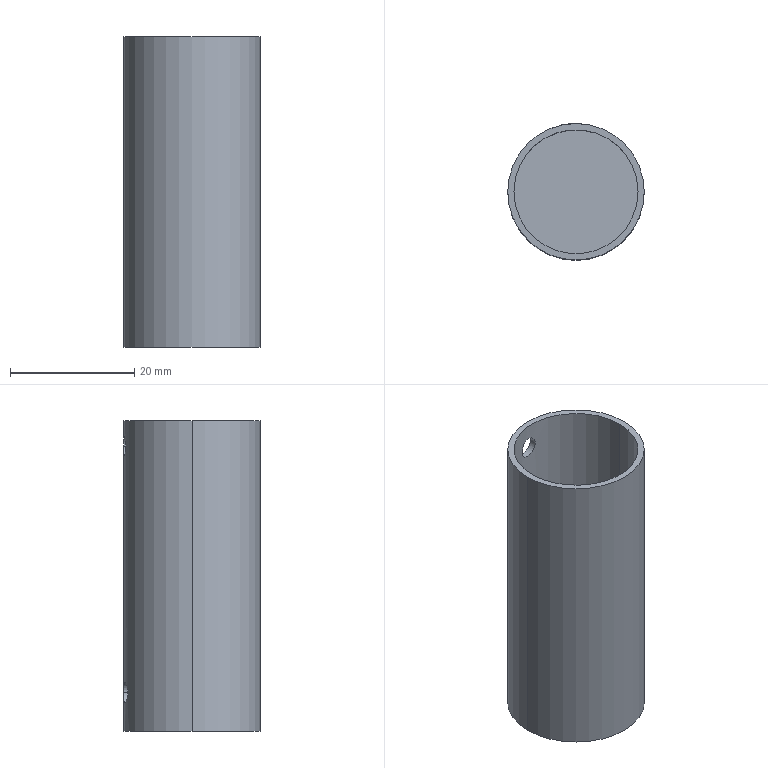Part | NX | 1 solid | 14 faces | box 22 x 22 x 50 mm | volume 4852 mm3 | cylinder 10 | plane 4 | commonest cylinder face diameters 3.3 x4 20 x4 22 x2
STEP:
#1=CARTESIAN_POINT('',(-0.2065,9.998,6.201));
#2=VERTEX_POINT('',#1);
#3=CARTESIAN_POINT('',(-3.449,9.386,6.201));
#4=VERTEX_POINT('',#3);
#5=CARTESIAN_POINT('',(-0.2065,9.998,6.201));
#6=CARTESIAN_POINT('',(-0.2065,9.998,6.018));
#7=CARTESIAN_POINT('',(-0.2384,9.997,5.832));
#8=CARTESIAN_POINT('',(-0.2992,9.996,5.659));
#9=CARTESIAN_POINT('',(-0.3601,9.994,5.486));
#10=CARTESIAN_POINT('',(-0.4514,9.99,5.322));
#11=CARTESIAN_POINT('',(-0.5654,9.984,5.178));
#12=CARTESIAN_POINT('',(-0.6803,9.977,5.034));
#13=CARTESIAN_POINT('',(-0.8214,9.967,4.907));
#14=CARTESIAN_POINT('',(-0.9768,9.952,4.808));
#15=CARTESIAN_POINT('',(-1.133,9.937,4.709));
#16=CARTESIAN_POINT('',(-1.308,9.916,4.635));
#17=CARTESIAN_POINT('',(-1.487,9.889,4.593));
#18=CARTESIAN_POINT('',(-1.665,9.862,4.552));
#19=CARTESIAN_POINT('',(-1.851,9.829,4.541));
#20=CARTESIAN_POINT('',(-2.03,9.792,4.561));
#21=CARTESIAN_POINT('',(-2.208,9.755,4.581));
#22=CARTESIAN_POINT('',(-2.383,9.713,4.632));
#23=CARTESIAN_POINT('',(-2.543,9.671,4.71));
#24=CARTESIAN_POINT('',(-2.703,9.629,4.788));
#25=CARTESIAN_POINT('',(-2.851,9.586,4.895));
#26=CARTESIAN_POINT('',(-2.977,9.547,5.023));
#27=CARTESIAN_POINT('',(-3.103,9.507,5.153));
#28=CARTESIAN_POINT('',(-3.21,9.471,5.307));
#29=CARTESIAN_POINT('',(-3.288,9.444,5.473));
#30=CARTESIAN_POINT('',(-3.366,9.417,5.639));
#31=CARTESIAN_POINT('',(-3.417,9.398,5.822));
#32=CARTESIAN_POINT('',(-3.438,9.39,6.006));
#33=CARTESIAN_POINT('',(-3.446,9.388,6.071));
#34=CARTESIAN_POINT('',(-3.449,9.386,6.136));
#35=CARTESIAN_POINT('',(-3.449,9.386,6.201));
#36=B_SPLINE_CURVE_WITH_KNOTS('',3,(#5,#6,#7,#8,#9,#10,#11,#12,#13,#14,#15,#16,#17,#18,#19,#20,#21,#22,#23,#24,#25,#26,#27,#28,#29,#30,#31,#32,#33,#34,#35),.UNSPECIFIED.,.F.,.F.,(4,3,3,3,3,3,3,3,3,3,4),(0.,0.1064,0.2128,0.3201,0.428,0.535,0.6409,0.7472,0.8549,0.9627,1.),.UNSPECIFIED.);
#37=EDGE_CURVE('',#2,#4,#36,.T.);
#38=ORIENTED_EDGE('',*,*,#37,.F.);
#39=CARTESIAN_POINT('',(-0.3942,10.993,6.201));
#40=VERTEX_POINT('',#39);
#41=CARTESIAN_POINT('',(-0.4173,11.115,6.201));
#42=DIRECTION('',(0.1853,-0.9827,0.));
#43=VECTOR('',#42,1.);
#44=LINE('',#41,#43);
#45=EDGE_CURVE('',#40,#2,#44,.T.);
#46=ORIENTED_EDGE('',*,*,#45,.F.);
#47=CARTESIAN_POINT('',(-3.637,10.381,6.201));
#48=VERTEX_POINT('',#47);
#49=CARTESIAN_POINT('',(-3.637,10.381,6.201));
#50=CARTESIAN_POINT('',(-3.637,10.381,6.017));
#51=CARTESIAN_POINT('',(-3.607,10.392,5.831));
#52=CARTESIAN_POINT('',(-3.549,10.412,5.658));
#53=CARTESIAN_POINT('',(-3.492,10.431,5.485));
#54=CARTESIAN_POINT('',(-3.405,10.46,5.32));
#55=CARTESIAN_POINT('',(-3.296,10.495,5.177));
#56=CARTESIAN_POINT('',(-3.186,10.529,5.032));
#57=CARTESIAN_POINT('',(-3.05,10.57,4.906));
#58=CARTESIAN_POINT('',(-2.9,10.611,4.807));
#59=CARTESIAN_POINT('',(-2.748,10.652,4.708));
#60=CARTESIAN_POINT('',(-2.577,10.695,4.634));
#61=CARTESIAN_POINT('',(-2.401,10.735,4.593));
#62=CARTESIAN_POINT('',(-2.226,10.774,4.552));
#63=CARTESIAN_POINT('',(-2.04,10.811,4.541));
#64=CARTESIAN_POINT('',(-1.859,10.842,4.561));
#65=CARTESIAN_POINT('',(-1.68,10.872,4.581));
#66=CARTESIAN_POINT('',(-1.501,10.898,4.633));
#67=CARTESIAN_POINT('',(-1.338,10.918,4.711));
#68=CARTESIAN_POINT('',(-1.173,10.939,4.79));
#69=CARTESIAN_POINT('',(-1.019,10.953,4.898));
#70=CARTESIAN_POINT('',(-0.8887,10.964,5.026));
#71=CARTESIAN_POINT('',(-0.7569,10.975,5.156));
#72=CARTESIAN_POINT('',(-0.6452,10.981,5.31));
#73=CARTESIAN_POINT('',(-0.5634,10.986,5.476));
#74=CARTESIAN_POINT('',(-0.4815,10.99,5.643));
#75=CARTESIAN_POINT('',(-0.4272,10.992,5.826));
#76=CARTESIAN_POINT('',(-0.4055,10.993,6.01));
#77=CARTESIAN_POINT('',(-0.398,10.993,6.073));
#78=CARTESIAN_POINT('',(-0.3942,10.993,6.137));
#79=CARTESIAN_POINT('',(-0.3942,10.993,6.201));
#80=B_SPLINE_CURVE_WITH_KNOTS('',3,(#49,#50,#51,#52,#53,#54,#55,#56,#57,#58,#59,#60,#61,#62,#63,#64,#65,#66,#67,#68,#69,#70,#71,#72,#73,#74,#75,#76,#77,#78,#79),.UNSPECIFIED.,.F.,.F.,(4,3,3,3,3,3,3,3,3,3,4),(0.,0.1066,0.2131,0.3205,0.4283,0.5353,0.6415,0.748,0.8557,0.9634,1.),.UNSPECIFIED.);
#81=EDGE_CURVE('',#48,#40,#80,.T.);
#82=ORIENTED_EDGE('',*,*,#81,.F.);
#83=CARTESIAN_POINT('',(-3.66,10.504,6.201));
#84=DIRECTION('',(0.1853,-0.9827,0.));
#85=VECTOR('',#84,1.);
#86=LINE('',#83,#85);
#87=EDGE_CURVE('',#48,#4,#86,.T.);
#88=ORIENTED_EDGE('',*,*,#87,.T.);
#89=EDGE_LOOP('',(#38,#46,#82,#88));
#90=FACE_OUTER_BOUND('',#89,.T.);
#91=CARTESIAN_POINT('',(-2.039,10.809,6.201));
#92=DIRECTION('',(-0.1853,0.9827,0.));
#93=DIRECTION('',(-0.9827,-0.1853,0.));
#94=AXIS2_PLACEMENT_3D('',#91,#92,#93);
#95=CYLINDRICAL_SURFACE('',#94,1.65);
#96=ADVANCED_FACE('',(#90),#95,.F.);
#97=CARTESIAN_POINT('',(0.6601,9.978,45.914));
#98=VERTEX_POINT('',#97);
#99=CARTESIAN_POINT('',(-2.624,9.65,45.914));
#100=VERTEX_POINT('',#99);
#101=CARTESIAN_POINT('',(0.6601,9.978,45.914));
#102=CARTESIAN_POINT('',(0.6601,9.978,45.731));
#103=CARTESIAN_POINT('',(0.6283,9.98,45.545));
#104=CARTESIAN_POINT('',(0.5675,9.984,45.372));
#105=CARTESIAN_POINT('',(0.5068,9.987,45.199));
#106=CARTESIAN_POINT('',(0.4155,9.992,45.034));
#107=CARTESIAN_POINT('',(0.3014,9.995,44.891));
#108=CARTESIAN_POINT('',(0.1863,9.999,44.747));
#109=CARTESIAN_POINT('',(0.0449,10.001,44.62));
#110=CARTESIAN_POINT('',(-0.1113,9.999,44.521));
#111=CARTESIAN_POINT('',(-0.2683,9.998,44.422));
#112=CARTESIAN_POINT('',(-0.4446,9.992,44.348));
#113=CARTESIAN_POINT('',(-0.6254,9.98,44.306));
#114=CARTESIAN_POINT('',(-0.8044,9.969,44.265));
#115=CARTESIAN_POINT('',(-0.9928,9.952,44.254));
#116=CARTESIAN_POINT('',(-1.175,9.931,44.274));
#117=CARTESIAN_POINT('',(-1.355,9.909,44.294));
#118=CARTESIAN_POINT('',(-1.533,9.883,44.345));
#119=CARTESIAN_POINT('',(-1.696,9.855,44.423));
#120=CARTESIAN_POINT('',(-1.859,9.827,44.501));
#121=CARTESIAN_POINT('',(-2.011,9.797,44.608));
#122=CARTESIAN_POINT('',(-2.139,9.769,44.736));
#123=CARTESIAN_POINT('',(-2.268,9.74,44.866));
#124=CARTESIAN_POINT('',(-2.378,9.714,45.02));
#125=CARTESIAN_POINT('',(-2.458,9.693,45.186));
#126=CARTESIAN_POINT('',(-2.538,9.673,45.352));
#127=CARTESIAN_POINT('',(-2.591,9.659,45.535));
#128=CARTESIAN_POINT('',(-2.612,9.653,45.719));
#129=CARTESIAN_POINT('',(-2.62,9.651,45.784));
#130=CARTESIAN_POINT('',(-2.624,9.65,45.849));
#131=CARTESIAN_POINT('',(-2.624,9.65,45.914));
#132=B_SPLINE_CURVE_WITH_KNOTS('',3,(#101,#102,#103,#104,#105,#106,#107,#108,#109,#110,#111,#112,#113,#114,#115,#116,#117,#118,#119,#120,#121,#122,#123,#124,#125,#126,#127,#128,#129,#130,#131),.UNSPECIFIED.,.F.,.F.,(4,3,3,3,3,3,3,3,3,3,4),(0.,0.1064,0.2128,0.3201,0.428,0.535,0.6409,0.7472,0.8549,0.9627,1.),.UNSPECIFIED.);
#133=EDGE_CURVE('',#98,#100,#132,.T.);
#134=ORIENTED_EDGE('',*,*,#133,.F.);
#135=CARTESIAN_POINT('',(0.5593,10.986,45.914));
#136=VERTEX_POINT('',#135);
#137=CARTESIAN_POINT('',(0.5469,11.11,45.914));
#138=DIRECTION('',(0.09954,-0.995,0.));
#139=VECTOR('',#138,1.);
#140=LINE('',#137,#139);
#141=EDGE_CURVE('',#136,#98,#140,.T.);
#142=ORIENTED_EDGE('',*,*,#141,.F.);
#143=CARTESIAN_POINT('',(-2.724,10.657,45.914));
#144=VERTEX_POINT('',#143);
#145=CARTESIAN_POINT('',(-2.724,10.657,45.914));
#146=CARTESIAN_POINT('',(-2.724,10.657,45.73));
#147=CARTESIAN_POINT('',(-2.693,10.665,45.544));
#148=CARTESIAN_POINT('',(-2.634,10.68,45.371));
#149=CARTESIAN_POINT('',(-2.575,10.694,45.198));
#150=CARTESIAN_POINT('',(-2.486,10.716,45.033));
#151=CARTESIAN_POINT('',(-2.375,10.741,44.89));
#152=CARTESIAN_POINT('',(-2.262,10.766,44.745));
#153=CARTESIAN_POINT('',(-2.124,10.794,44.619));
#154=CARTESIAN_POINT('',(-1.97,10.822,44.52));
#155=CARTESIAN_POINT('',(-1.815,10.85,44.421));
#156=CARTESIAN_POINT('',(-1.641,10.878,44.347));
#157=CARTESIAN_POINT('',(-1.462,10.902,44.306));
#158=CARTESIAN_POINT('',(-1.284,10.926,44.265));
#159=CARTESIAN_POINT('',(-1.096,10.947,44.254));
#160=CARTESIAN_POINT('',(-0.9135,10.962,44.274));
#161=CARTESIAN_POINT('',(-0.7325,10.977,44.294));
#162=CARTESIAN_POINT('',(-0.552,10.987,44.346));
#163=CARTESIAN_POINT('',(-0.387,10.993,44.424));
#164=CARTESIAN_POINT('',(-0.2214,10.999,44.503));
#165=CARTESIAN_POINT('',(-0.06681,11.001,44.611));
#166=CARTESIAN_POINT('',(0.06417,11.,44.739));
#167=CARTESIAN_POINT('',(0.1964,10.999,44.869));
#168=CARTESIAN_POINT('',(0.3082,10.996,45.023));
#169=CARTESIAN_POINT('',(0.3901,10.993,45.189));
#170=CARTESIAN_POINT('',(0.4721,10.99,45.356));
#171=CARTESIAN_POINT('',(0.5264,10.987,45.539));
#172=CARTESIAN_POINT('',(0.5481,10.986,45.723));
#173=CARTESIAN_POINT('',(0.5555,10.986,45.786));
#174=CARTESIAN_POINT('',(0.5593,10.986,45.85));
#175=CARTESIAN_POINT('',(0.5593,10.986,45.914));
#176=B_SPLINE_CURVE_WITH_KNOTS('',3,(#145,#146,#147,#148,#149,#150,#151,#152,#153,#154,#155,#156,#157,#158,#159,#160,#161,#162,#163,#164,#165,#166,#167,#168,#169,#170,#171,#172,#173,#174,#175),.UNSPECIFIED.,.F.,.F.,(4,3,3,3,3,3,3,3,3,3,4),(0.,0.1066,0.2131,0.3205,0.4283,0.5353,0.6415,0.748,0.8557,0.9634,1.),.UNSPECIFIED.);
#177=EDGE_CURVE('',#144,#136,#176,.T.);
#178=ORIENTED_EDGE('',*,*,#177,.F.);
#179=CARTESIAN_POINT('',(-2.737,10.781,45.914));
#180=DIRECTION('',(0.09954,-0.995,0.));
#181=VECTOR('',#180,1.);
#182=LINE('',#179,#181);
#183=EDGE_CURVE('',#144,#100,#182,.T.);
#184=ORIENTED_EDGE('',*,*,#183,.T.);
#185=EDGE_LOOP('',(#134,#142,#178,#184));
#186=FACE_OUTER_BOUND('',#185,.T.);
#187=CARTESIAN_POINT('',(-1.095,10.945,45.914));
#188=DIRECTION('',(-0.09954,0.995,0.));
#189=DIRECTION('',(-0.995,-0.09954,0.));
#190=AXIS2_PLACEMENT_3D('',#187,#188,#189);
#191=CYLINDRICAL_SURFACE('',#190,1.65);
#192=ADVANCED_FACE('',(#186),#191,.F.);
#193=CARTESIAN_POINT('',(10.,0.,25.));
#194=VERTEX_POINT('',#193);
#195=CARTESIAN_POINT('',(-10.,0.,25.));
#196=VERTEX_POINT('',#195);
#197=CARTESIAN_POINT('',(0.,0.,25.));
#198=DIRECTION('',(0.,0.,-1.));
#199=DIRECTION('',(-1.,0.,0.));
#200=AXIS2_PLACEMENT_3D('',#197,#198,#199);
#201=CIRCLE('',#200,10.);
#202=EDGE_CURVE('',#194,#196,#201,.T.);
#203=ORIENTED_EDGE('',*,*,#202,.F.);
#204=CARTESIAN_POINT('',(10.,0.,0.));
#205=VERTEX_POINT('',#204);
#206=CARTESIAN_POINT('',(10.,0.,25.));
#207=DIRECTION('',(0.,0.,1.));
#208=VECTOR('',#207,1.);
#209=LINE('',#206,#208);
#210=EDGE_CURVE('',#205,#194,#209,.T.);
#211=ORIENTED_EDGE('',*,*,#210,.F.);
#212=CARTESIAN_POINT('',(-10.,0.,0.));
#213=VERTEX_POINT('',#212);
#214=CARTESIAN_POINT('',(0.,0.,0.));
#215=DIRECTION('',(0.,0.,-1.));
#216=DIRECTION('',(-1.,0.,0.));
#217=AXIS2_PLACEMENT_3D('',#214,#215,#216);
#218=CIRCLE('',#217,10.);
#219=EDGE_CURVE('',#205,#213,#218,.T.);
#220=ORIENTED_EDGE('',*,*,#219,.T.);
#221=CARTESIAN_POINT('',(-10.,0.,25.));
#222=DIRECTION('',(0.,0.,1.));
#223=VECTOR('',#222,1.);
#224=LINE('',#221,#223);
#225=EDGE_CURVE('',#213,#196,#224,.T.);
#226=ORIENTED_EDGE('',*,*,#225,.T.);
#227=EDGE_LOOP('',(#203,#211,#220,#226));
#228=FACE_OUTER_BOUND('',#227,.T.);
#229=CARTESIAN_POINT('',(0.,0.,25.));
#230=DIRECTION('',(0.,0.,-1.));
#231=DIRECTION('',(-1.,0.,0.));
#232=AXIS2_PLACEMENT_3D('',#229,#230,#231);
#233=CYLINDRICAL_SURFACE('',#232,10.);
#234=ADVANCED_FACE('',(#228),#233,.F.);
#235=CARTESIAN_POINT('',(-10.,0.,30.));
#236=VERTEX_POINT('',#235);
#237=CARTESIAN_POINT('',(10.,0.,30.));
#238=VERTEX_POINT('',#237);
#239=CARTESIAN_POINT('',(0.,0.,30.));
#240=DIRECTION('',(0.,0.,1.));
#241=DIRECTION('',(1.,0.,0.));
#242=AXIS2_PLACEMENT_3D('',#239,#240,#241);
#243=CIRCLE('',#242,10.);
#244=EDGE_CURVE('',#236,#238,#243,.T.);
#245=ORIENTED_EDGE('',*,*,#244,.F.);
#246=CARTESIAN_POINT('',(-10.,0.,50.));
#247=VERTEX_POINT('',#246);
#248=CARTESIAN_POINT('',(-10.,0.,30.));
#249=DIRECTION('',(0.,0.,1.));
#250=VECTOR('',#249,1.);
#251=LINE('',#248,#250);
#252=EDGE_CURVE('',#236,#247,#251,.T.);
#253=ORIENTED_EDGE('',*,*,#252,.T.);
#254=CARTESIAN_POINT('',(10.,0.,50.));
#255=VERTEX_POINT('',#254);
#256=CARTESIAN_POINT('',(0.,0.,50.));
#257=DIRECTION('',(0.,0.,1.));
#258=DIRECTION('',(1.,0.,0.));
#259=AXIS2_PLACEMENT_3D('',#256,#257,#258);
#260=CIRCLE('',#259,10.);
#261=EDGE_CURVE('',#247,#255,#260,.T.);
#262=ORIENTED_EDGE('',*,*,#261,.T.);
#263=CARTESIAN_POINT('',(10.,0.,30.));
#264=DIRECTION('',(0.,0.,1.));
#265=VECTOR('',#264,1.);
#266=LINE('',#263,#265);
#267=EDGE_CURVE('',#238,#255,#266,.T.);
#268=ORIENTED_EDGE('',*,*,#267,.F.);
#269=EDGE_LOOP('',(#245,#253,#262,#268));
#270=FACE_OUTER_BOUND('',#269,.T.);
#271=CARTESIAN_POINT('',(0.,0.,30.));
#272=DIRECTION('',(0.,0.,1.));
#273=DIRECTION('',(1.,0.,0.));
#274=AXIS2_PLACEMENT_3D('',#271,#272,#273);
#275=CYLINDRICAL_SURFACE('',#274,10.);
#276=ADVANCED_FACE('',(#270),#275,.F.);
#277=ORIENTED_EDGE('',*,*,#81,.T.);
#278=CARTESIAN_POINT('',(-0.3942,10.993,6.201));
#279=CARTESIAN_POINT('',(-0.3942,10.993,6.385));
#280=CARTESIAN_POINT('',(-0.4261,10.992,6.571));
#281=CARTESIAN_POINT('',(-0.4869,10.989,6.744));
#282=CARTESIAN_POINT('',(-0.5477,10.987,6.917));
#283=CARTESIAN_POINT('',(-0.6391,10.982,7.082));
#284=CARTESIAN_POINT('',(-0.7532,10.974,7.225));
#285=CARTESIAN_POINT('',(-0.8681,10.966,7.37));
#286=CARTESIAN_POINT('',(-1.009,10.955,7.496));
#287=CARTESIAN_POINT('',(-1.165,10.938,7.595));
#288=CARTESIAN_POINT('',(-1.321,10.922,7.694));
#289=CARTESIAN_POINT('',(-1.496,10.899,7.768));
#290=CARTESIAN_POINT('',(-1.674,10.872,7.809));
#291=CARTESIAN_POINT('',(-1.852,10.844,7.85));
#292=CARTESIAN_POINT('',(-2.038,10.811,7.861));
#293=CARTESIAN_POINT('',(-2.217,10.774,7.841));
#294=CARTESIAN_POINT('',(-2.395,10.738,7.821));
#295=CARTESIAN_POINT('',(-2.571,10.697,7.769));
#296=CARTESIAN_POINT('',(-2.731,10.656,7.691));
#297=CARTESIAN_POINT('',(-2.892,10.614,7.612));
#298=CARTESIAN_POINT('',(-3.041,10.572,7.504));
#299=CARTESIAN_POINT('',(-3.166,10.535,7.376));
#300=CARTESIAN_POINT('',(-3.293,10.496,7.246));
#301=CARTESIAN_POINT('',(-3.399,10.462,7.092));
#302=CARTESIAN_POINT('',(-3.477,10.436,6.926));
#303=CARTESIAN_POINT('',(-3.555,10.41,6.759));
#304=CARTESIAN_POINT('',(-3.606,10.392,6.576));
#305=CARTESIAN_POINT('',(-3.626,10.385,6.392));
#306=CARTESIAN_POINT('',(-3.633,10.383,6.329));
#307=CARTESIAN_POINT('',(-3.637,10.381,6.265));
#308=CARTESIAN_POINT('',(-3.637,10.381,6.201));
#309=B_SPLINE_CURVE_WITH_KNOTS('',3,(#278,#279,#280,#281,#282,#283,#284,#285,#286,#287,#288,#289,#290,#291,#292,#293,#294,#295,#296,#297,#298,#299,#300,#301,#302,#303,#304,#305,#306,#307,#308),.UNSPECIFIED.,.F.,.F.,(4,3,3,3,3,3,3,3,3,3,4),(0.,0.1066,0.2131,0.3205,0.4283,0.5353,0.6415,0.748,0.8557,0.9634,1.),.UNSPECIFIED.);
#310=EDGE_CURVE('',#40,#48,#309,.T.);
#311=ORIENTED_EDGE('',*,*,#310,.T.);
#312=EDGE_LOOP('',(#277,#311));
#313=FACE_BOUND('',#312,.T.);
#314=ORIENTED_EDGE('',*,*,#177,.T.);
#315=CARTESIAN_POINT('',(0.5593,10.986,45.914));
#316=CARTESIAN_POINT('',(0.5593,10.986,46.097));
#317=CARTESIAN_POINT('',(0.5275,10.988,46.283));
#318=CARTESIAN_POINT('',(0.4666,10.99,46.457));
#319=CARTESIAN_POINT('',(0.4058,10.993,46.63));
#320=CARTESIAN_POINT('',(0.3143,10.996,46.795));
#321=CARTESIAN_POINT('',(0.2,10.998,46.938));
#322=CARTESIAN_POINT('',(0.08485,11.,47.082));
#323=CARTESIAN_POINT('',(-0.05668,11.001,47.209));
#324=CARTESIAN_POINT('',(-0.2129,10.998,47.308));
#325=CARTESIAN_POINT('',(-0.3698,10.995,47.407));
#326=CARTESIAN_POINT('',(-0.546,10.988,47.48));
#327=CARTESIAN_POINT('',(-0.7265,10.976,47.522));
#328=CARTESIAN_POINT('',(-0.9057,10.964,47.563));
#329=CARTESIAN_POINT('',(-1.094,10.947,47.574));
#330=CARTESIAN_POINT('',(-1.276,10.926,47.554));
#331=CARTESIAN_POINT('',(-1.456,10.905,47.534));
#332=CARTESIAN_POINT('',(-1.635,10.879,47.482));
#333=CARTESIAN_POINT('',(-1.798,10.852,47.404));
#334=CARTESIAN_POINT('',(-1.962,10.825,47.325));
#335=CARTESIAN_POINT('',(-2.114,10.796,47.217));
#336=CARTESIAN_POINT('',(-2.242,10.769,47.089));
#337=CARTESIAN_POINT('',(-2.371,10.742,46.959));
#338=CARTESIAN_POINT('',(-2.48,10.717,46.805));
#339=CARTESIAN_POINT('',(-2.56,10.698,46.638));
#340=CARTESIAN_POINT('',(-2.64,10.679,46.472));
#341=CARTESIAN_POINT('',(-2.692,10.665,46.289));
#342=CARTESIAN_POINT('',(-2.713,10.66,46.105));
#343=CARTESIAN_POINT('',(-2.721,10.658,46.042));
#344=CARTESIAN_POINT('',(-2.724,10.657,45.978));
#345=CARTESIAN_POINT('',(-2.724,10.657,45.914));
#346=B_SPLINE_CURVE_WITH_KNOTS('',3,(#315,#316,#317,#318,#319,#320,#321,#322,#323,#324,#325,#326,#327,#328,#329,#330,#331,#332,#333,#334,#335,#336,#337,#338,#339,#340,#341,#342,#343,#344,#345),.UNSPECIFIED.,.F.,.F.,(4,3,3,3,3,3,3,3,3,3,4),(0.,0.1066,0.2131,0.3205,0.4283,0.5353,0.6415,0.748,0.8557,0.9634,1.),.UNSPECIFIED.);
#347=EDGE_CURVE('',#136,#144,#346,.T.);
#348=ORIENTED_EDGE('',*,*,#347,.T.);
#349=EDGE_LOOP('',(#314,#348));
#350=FACE_BOUND('',#349,.T.);
#351=CARTESIAN_POINT('',(11.,0.,50.));
#352=VERTEX_POINT('',#351);
#353=CARTESIAN_POINT('',(-11.,0.,50.));
#354=VERTEX_POINT('',#353);
#355=CARTESIAN_POINT('',(0.,0.,50.));
#356=DIRECTION('',(0.,0.,1.));
#357=DIRECTION('',(1.,0.,0.));
#358=AXIS2_PLACEMENT_3D('',#355,#356,#357);
#359=CIRCLE('',#358,11.);
#360=EDGE_CURVE('',#352,#354,#359,.T.);
#361=ORIENTED_EDGE('',*,*,#360,.F.);
#362=CARTESIAN_POINT('',(11.,0.,0.));
#363=VERTEX_POINT('',#362);
#364=CARTESIAN_POINT('',(11.,0.,50.));
#365=DIRECTION('',(0.,0.,1.));
#366=VECTOR('',#365,1.);
#367=LINE('',#364,#366);
#368=EDGE_CURVE('',#363,#352,#367,.T.);
#369=ORIENTED_EDGE('',*,*,#368,.F.);
#370=CARTESIAN_POINT('',(-11.,0.,0.));
#371=VERTEX_POINT('',#370);
#372=CARTESIAN_POINT('',(0.,0.,0.));
#373=DIRECTION('',(0.,0.,1.));
#374=DIRECTION('',(1.,0.,0.));
#375=AXIS2_PLACEMENT_3D('',#372,#373,#374);
#376=CIRCLE('',#375,11.);
#377=EDGE_CURVE('',#363,#371,#376,.T.);
#378=ORIENTED_EDGE('',*,*,#377,.T.);
#379=CARTESIAN_POINT('',(-11.,0.,50.));
#380=DIRECTION('',(0.,0.,1.));
#381=VECTOR('',#380,1.);
#382=LINE('',#379,#381);
#383=EDGE_CURVE('',#371,#354,#382,.T.);
#384=ORIENTED_EDGE('',*,*,#383,.T.);
#385=EDGE_LOOP('',(#361,#369,#378,#384));
#386=FACE_BOUND('',#385,.T.);
#387=CARTESIAN_POINT('',(0.,0.,50.));
#388=DIRECTION('',(0.,0.,-1.));
#389=DIRECTION('',(-1.,0.,0.));
#390=AXIS2_PLACEMENT_3D('',#387,#388,#389);
#391=CYLINDRICAL_SURFACE('',#390,11.);
#392=ADVANCED_FACE('',(#313,#350,#386),#391,.T.);
#393=ORIENTED_EDGE('',*,*,#368,.T.);
#394=CARTESIAN_POINT('',(0.,0.,50.));
#395=DIRECTION('',(0.,0.,1.));
#396=DIRECTION('',(1.,0.,0.));
#397=AXIS2_PLACEMENT_3D('',#394,#395,#396);
#398=CIRCLE('',#397,11.);
#399=EDGE_CURVE('',#354,#352,#398,.T.);
#400=ORIENTED_EDGE('',*,*,#399,.F.);
#401=ORIENTED_EDGE('',*,*,#383,.F.);
#402=CARTESIAN_POINT('',(0.,0.,0.));
#403=DIRECTION('',(0.,0.,1.));
#404=DIRECTION('',(1.,0.,0.));
#405=AXIS2_PLACEMENT_3D('',#402,#403,#404);
#406=CIRCLE('',#405,11.);
#407=EDGE_CURVE('',#371,#363,#406,.T.);
#408=ORIENTED_EDGE('',*,*,#407,.T.);
#409=EDGE_LOOP('',(#393,#400,#401,#408));
#410=FACE_OUTER_BOUND('',#409,.T.);
#411=CARTESIAN_POINT('',(0.,0.,50.));
#412=DIRECTION('',(0.,0.,-1.));
#413=DIRECTION('',(-1.,0.,0.));
#414=AXIS2_PLACEMENT_3D('',#411,#412,#413);
#415=CYLINDRICAL_SURFACE('',#414,11.);
#416=ADVANCED_FACE('',(#410),#415,.T.);
#417=CARTESIAN_POINT('',(0.,0.,50.));
#418=DIRECTION('',(0.,0.,1.));
#419=DIRECTION('',(1.,0.,0.));
#420=AXIS2_PLACEMENT_3D('',#417,#418,#419);
#421=CIRCLE('',#420,10.);
#422=EDGE_CURVE('',#255,#247,#421,.T.);
#423=ORIENTED_EDGE('',*,*,#422,.F.);
#424=ORIENTED_EDGE('',*,*,#261,.F.);
#425=EDGE_LOOP('',(#423,#424));
#426=FACE_BOUND('',#425,.T.);
#427=ORIENTED_EDGE('',*,*,#399,.T.);
#428=ORIENTED_EDGE('',*,*,#360,.T.);
#429=EDGE_LOOP('',(#427,#428));
#430=FACE_BOUND('',#429,.T.);
#431=CARTESIAN_POINT('',(0.,0.,50.));
#432=DIRECTION('',(0.,0.,1.));
#433=DIRECTION('',(1.,0.,0.));
#434=AXIS2_PLACEMENT_3D('',#431,#432,#433);
#435=PLANE('',#434);
#436=ADVANCED_FACE('',(#426,#430),#435,.T.);
#437=CARTESIAN_POINT('',(0.,0.,0.));
#438=DIRECTION('',(0.,0.,-1.));
#439=DIRECTION('',(-1.,0.,0.));
#440=AXIS2_PLACEMENT_3D('',#437,#438,#439);
#441=CIRCLE('',#440,10.);
#442=EDGE_CURVE('',#213,#205,#441,.T.);
#443=ORIENTED_EDGE('',*,*,#442,.F.);
#444=ORIENTED_EDGE('',*,*,#219,.F.);
#445=EDGE_LOOP('',(#443,#444));
#446=FACE_BOUND('',#445,.T.);
#447=ORIENTED_EDGE('',*,*,#407,.F.);
#448=ORIENTED_EDGE('',*,*,#377,.F.);
#449=EDGE_LOOP('',(#447,#448));
#450=FACE_BOUND('',#449,.T.);
#451=CARTESIAN_POINT('',(0.,0.,0.));
#452=DIRECTION('',(0.,0.,1.));
#453=DIRECTION('',(1.,0.,0.));
#454=AXIS2_PLACEMENT_3D('',#451,#452,#453);
#455=PLANE('',#454);
#456=ADVANCED_FACE('',(#446,#450),#455,.F.);
#457=ORIENTED_EDGE('',*,*,#252,.F.);
#458=CARTESIAN_POINT('',(0.,0.,30.));
#459=DIRECTION('',(0.,0.,1.));
#460=DIRECTION('',(1.,0.,0.));
#461=AXIS2_PLACEMENT_3D('',#458,#459,#460);
#462=CIRCLE('',#461,10.);
#463=EDGE_CURVE('',#238,#236,#462,.T.);
#464=ORIENTED_EDGE('',*,*,#463,.F.);
#465=ORIENTED_EDGE('',*,*,#267,.T.);
#466=ORIENTED_EDGE('',*,*,#422,.T.);
#467=EDGE_LOOP('',(#457,#464,#465,#466));
#468=FACE_BOUND('',#467,.T.);
#469=CARTESIAN_POINT('',(-2.624,9.65,45.914));
#470=CARTESIAN_POINT('',(-2.624,9.65,46.097));
#471=CARTESIAN_POINT('',(-2.593,9.658,46.283));
#472=CARTESIAN_POINT('',(-2.534,9.674,46.456));
#473=CARTESIAN_POINT('',(-2.475,9.689,46.629));
#474=CARTESIAN_POINT('',(-2.387,9.712,46.793));
#475=CARTESIAN_POINT('',(-2.275,9.738,46.937));
#476=CARTESIAN_POINT('',(-2.163,9.764,47.081));
#477=CARTESIAN_POINT('',(-2.025,9.794,47.208));
#478=CARTESIAN_POINT('',(-1.872,9.823,47.307));
#479=CARTESIAN_POINT('',(-1.717,9.853,47.406));
#480=CARTESIAN_POINT('',(-1.543,9.882,47.48));
#481=CARTESIAN_POINT('',(-1.364,9.907,47.522));
#482=CARTESIAN_POINT('',(-1.186,9.931,47.563));
#483=CARTESIAN_POINT('',(-0.9982,9.952,47.574));
#484=CARTESIAN_POINT('',(-0.8158,9.967,47.554));
#485=CARTESIAN_POINT('',(-0.6351,9.981,47.534));
#486=CARTESIAN_POINT('',(-0.4549,9.991,47.483));
#487=CARTESIAN_POINT('',(-0.2901,9.996,47.405));
#488=CARTESIAN_POINT('',(-0.1245,10.001,47.327));
#489=CARTESIAN_POINT('',(0.03012,10.001,47.219));
#490=CARTESIAN_POINT('',(0.1613,9.999,47.092));
#491=CARTESIAN_POINT('',(0.294,9.997,46.962));
#492=CARTESIAN_POINT('',(0.4064,9.992,46.808));
#493=CARTESIAN_POINT('',(0.4888,9.988,46.642));
#494=CARTESIAN_POINT('',(0.5714,9.984,46.476));
#495=CARTESIAN_POINT('',(0.6262,9.98,46.293));
#496=CARTESIAN_POINT('',(0.6484,9.979,46.109));
#497=CARTESIAN_POINT('',(0.6562,9.978,46.044));
#498=CARTESIAN_POINT('',(0.6601,9.978,45.979));
#499=CARTESIAN_POINT('',(0.6601,9.978,45.914));
#500=B_SPLINE_CURVE_WITH_KNOTS('',3,(#469,#470,#471,#472,#473,#474,#475,#476,#477,#478,#479,#480,#481,#482,#483,#484,#485,#486,#487,#488,#489,#490,#491,#492,#493,#494,#495,#496,#497,#498,#499),.UNSPECIFIED.,.F.,.F.,(4,3,3,3,3,3,3,3,3,3,4),(0.,0.1064,0.2128,0.3201,0.428,0.535,0.6409,0.7472,0.8549,0.9627,1.),.UNSPECIFIED.);
#501=EDGE_CURVE('',#100,#98,#500,.T.);
#502=ORIENTED_EDGE('',*,*,#501,.T.);
#503=ORIENTED_EDGE('',*,*,#133,.T.);
#504=EDGE_LOOP('',(#502,#503));
#505=FACE_BOUND('',#504,.T.);
#506=CARTESIAN_POINT('',(0.,0.,30.));
#507=DIRECTION('',(0.,0.,1.));
#508=DIRECTION('',(1.,0.,0.));
#509=AXIS2_PLACEMENT_3D('',#506,#507,#508);
#510=CYLINDRICAL_SURFACE('',#509,10.);
#511=ADVANCED_FACE('',(#468,#505),#510,.F.);
#512=ORIENTED_EDGE('',*,*,#463,.T.);
#513=ORIENTED_EDGE('',*,*,#244,.T.);
#514=EDGE_LOOP('',(#512,#513));
#515=FACE_OUTER_BOUND('',#514,.T.);
#516=CARTESIAN_POINT('',(0.,0.,30.));
#517=DIRECTION('',(0.,0.,1.));
#518=DIRECTION('',(1.,0.,0.));
#519=AXIS2_PLACEMENT_3D('',#516,#517,#518);
#520=PLANE('',#519);
#521=ADVANCED_FACE('',(#515),#520,.T.);
#522=ORIENTED_EDGE('',*,*,#210,.T.);
#523=CARTESIAN_POINT('',(0.,0.,25.));
#524=DIRECTION('',(0.,0.,-1.));
#525=DIRECTION('',(-1.,0.,0.));
#526=AXIS2_PLACEMENT_3D('',#523,#524,#525);
#527=CIRCLE('',#526,10.);
#528=EDGE_CURVE('',#196,#194,#527,.T.);
#529=ORIENTED_EDGE('',*,*,#528,.F.);
#530=ORIENTED_EDGE('',*,*,#225,.F.);
#531=ORIENTED_EDGE('',*,*,#442,.T.);
#532=EDGE_LOOP('',(#522,#529,#530,#531));
#533=FACE_BOUND('',#532,.T.);
#534=CARTESIAN_POINT('',(-3.449,9.386,6.201));
#535=CARTESIAN_POINT('',(-3.449,9.386,6.384));
#536=CARTESIAN_POINT('',(-3.419,9.397,6.57));
#537=CARTESIAN_POINT('',(-3.362,9.418,6.743));
#538=CARTESIAN_POINT('',(-3.305,9.438,6.916));
#539=CARTESIAN_POINT('',(-3.219,9.469,7.08));
#540=CARTESIAN_POINT('',(-3.11,9.504,7.224));
#541=CARTESIAN_POINT('',(-3.001,9.54,7.368));
#542=CARTESIAN_POINT('',(-2.866,9.582,7.495));
#543=CARTESIAN_POINT('',(-2.715,9.624,7.594));
#544=CARTESIAN_POINT('',(-2.564,9.667,7.693));
#545=CARTESIAN_POINT('',(-2.393,9.711,7.767));
#546=CARTESIAN_POINT('',(-2.217,9.751,7.809));
#547=CARTESIAN_POINT('',(-2.042,9.791,7.85));
#548=CARTESIAN_POINT('',(-1.856,9.828,7.861));
#549=CARTESIAN_POINT('',(-1.676,9.859,7.841));
#550=CARTESIAN_POINT('',(-1.497,9.889,7.821));
#551=CARTESIAN_POINT('',(-1.318,9.914,7.77));
#552=CARTESIAN_POINT('',(-1.155,9.933,7.692));
#553=CARTESIAN_POINT('',(-0.9901,9.952,7.614));
#554=CARTESIAN_POINT('',(-0.8361,9.966,7.507));
#555=CARTESIAN_POINT('',(-0.7052,9.975,7.379));
#556=CARTESIAN_POINT('',(-0.5728,9.984,7.249));
#557=CARTESIAN_POINT('',(-0.4605,9.99,7.095));
#558=CARTESIAN_POINT('',(-0.378,9.993,6.929));
#559=CARTESIAN_POINT('',(-0.2954,9.996,6.763));
#560=CARTESIAN_POINT('',(-0.2405,9.997,6.58));
#561=CARTESIAN_POINT('',(-0.2183,9.998,6.396));
#562=CARTESIAN_POINT('',(-0.2105,9.998,6.331));
#563=CARTESIAN_POINT('',(-0.2065,9.998,6.266));
#564=CARTESIAN_POINT('',(-0.2065,9.998,6.201));
#565=B_SPLINE_CURVE_WITH_KNOTS('',3,(#534,#535,#536,#537,#538,#539,#540,#541,#542,#543,#544,#545,#546,#547,#548,#549,#550,#551,#552,#553,#554,#555,#556,#557,#558,#559,#560,#561,#562,#563,#564),.UNSPECIFIED.,.F.,.F.,(4,3,3,3,3,3,3,3,3,3,4),(0.,0.1064,0.2128,0.3201,0.428,0.535,0.6409,0.7472,0.8549,0.9627,1.),.UNSPECIFIED.);
#566=EDGE_CURVE('',#4,#2,#565,.T.);
#567=ORIENTED_EDGE('',*,*,#566,.T.);
#568=ORIENTED_EDGE('',*,*,#37,.T.);
#569=EDGE_LOOP('',(#567,#568));
#570=FACE_BOUND('',#569,.T.);
#571=CARTESIAN_POINT('',(0.,0.,25.));
#572=DIRECTION('',(0.,0.,-1.));
#573=DIRECTION('',(-1.,0.,0.));
#574=AXIS2_PLACEMENT_3D('',#571,#572,#573);
#575=CYLINDRICAL_SURFACE('',#574,10.);
#576=ADVANCED_FACE('',(#533,#570),#575,.F.);
#577=ORIENTED_EDGE('',*,*,#528,.T.);
#578=ORIENTED_EDGE('',*,*,#202,.T.);
#579=EDGE_LOOP('',(#577,#578));
#580=FACE_OUTER_BOUND('',#579,.T.);
#581=CARTESIAN_POINT('',(0.,0.,25.));
#582=DIRECTION('',(0.,0.,-1.));
#583=DIRECTION('',(-1.,0.,0.));
#584=AXIS2_PLACEMENT_3D('',#581,#582,#583);
#585=PLANE('',#584);
#586=ADVANCED_FACE('',(#580),#585,.T.);
#587=ORIENTED_EDGE('',*,*,#141,.T.);
#588=ORIENTED_EDGE('',*,*,#501,.F.);
#589=ORIENTED_EDGE('',*,*,#183,.F.);
#590=ORIENTED_EDGE('',*,*,#347,.F.);
#591=EDGE_LOOP('',(#587,#588,#589,#590));
#592=FACE_OUTER_BOUND('',#591,.T.);
#593=CARTESIAN_POINT('',(-1.095,10.945,45.914));
#594=DIRECTION('',(-0.09954,0.995,0.));
#595=DIRECTION('',(-0.995,-0.09954,0.));
#596=AXIS2_PLACEMENT_3D('',#593,#594,#595);
#597=CYLINDRICAL_SURFACE('',#596,1.65);
#598=ADVANCED_FACE('',(#592),#597,.F.);
#599=ORIENTED_EDGE('',*,*,#45,.T.);
#600=ORIENTED_EDGE('',*,*,#566,.F.);
#601=ORIENTED_EDGE('',*,*,#87,.F.);
#602=ORIENTED_EDGE('',*,*,#310,.F.);
#603=EDGE_LOOP('',(#599,#600,#601,#602));
#604=FACE_OUTER_BOUND('',#603,.T.);
#605=CARTESIAN_POINT('',(-2.039,10.809,6.201));
#606=DIRECTION('',(-0.1853,0.9827,0.));
#607=DIRECTION('',(-0.9827,-0.1853,0.));
#608=AXIS2_PLACEMENT_3D('',#605,#606,#607);
#609=CYLINDRICAL_SURFACE('',#608,1.65);
#610=ADVANCED_FACE('',(#604),#609,.F.);
#611=CLOSED_SHELL('',(#96,#192,#234,#276,#392,#416,#436,#456,#511,#521,#576,#586,#598,#610));
#612=MANIFOLD_SOLID_BREP('',#611);
#613=(LENGTH_UNIT()NAMED_UNIT(*)SI_UNIT(.MILLI.,.METRE.));
#614=UNCERTAINTY_MEASURE_WITH_UNIT(LENGTH_MEASURE(0.0508),#613,'','');
#615=(NAMED_UNIT(*)PLANE_ANGLE_UNIT()SI_UNIT($,.RADIAN.));
#616=PLANE_ANGLE_MEASURE_WITH_UNIT(PLANE_ANGLE_MEASURE(0.01745),#615);
#617=DIMENSIONAL_EXPONENTS(0.,0.,0.,0.,0.,0.,0.);
#618=(CONVERSION_BASED_UNIT('DEGREE',#616)NAMED_UNIT(#617)PLANE_ANGLE_UNIT());
#619=(NAMED_UNIT(*)SI_UNIT($,.STERADIAN.)SOLID_ANGLE_UNIT());
#620=(GEOMETRIC_REPRESENTATION_CONTEXT(3)GLOBAL_UNCERTAINTY_ASSIGNED_CONTEXT((#614))GLOBAL_UNIT_ASSIGNED_CONTEXT((#613,#618,#619))REPRESENTATION_CONTEXT('',''));
#621=ADVANCED_BREP_SHAPE_REPRESENTATION('',(#612),#620);